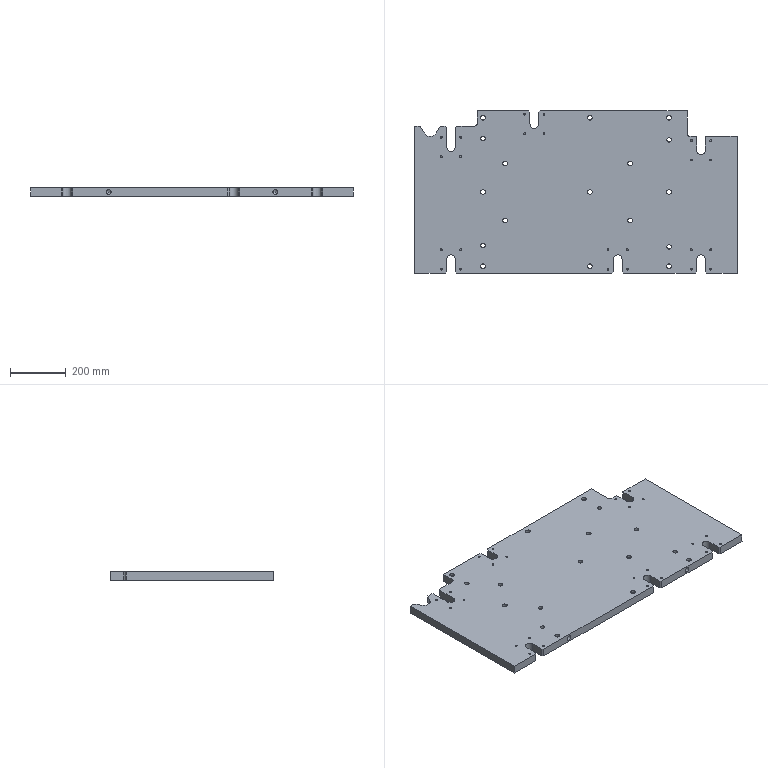Part | STEP file | 1 solid | 149 faces | box 1160 x 585 x 30 mm | volume 18789042 mm3 | cylinder 67 | plane 54 | cone 28 | commonest cylinder face diameters 6.8 x24 17 x13 26 x13 32 x6 16 x4 17.5 x4